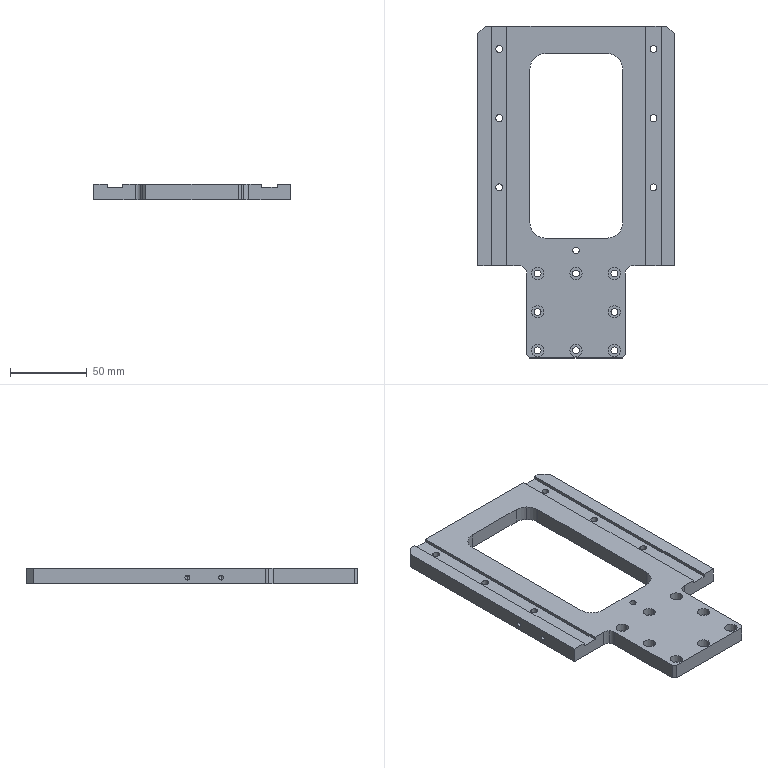Part | STEP file | ASND-0110-Body 1-17 | 1 solid | 122 faces | box 128 x 216 x 10 mm | volume 155040 mm3 | cylinder 78 | plane 40 | cone 4 | commonest cylinder face diameters 4.5 x28 8 x28 3.242 x8 20 x8 10 x4 4.134 x2